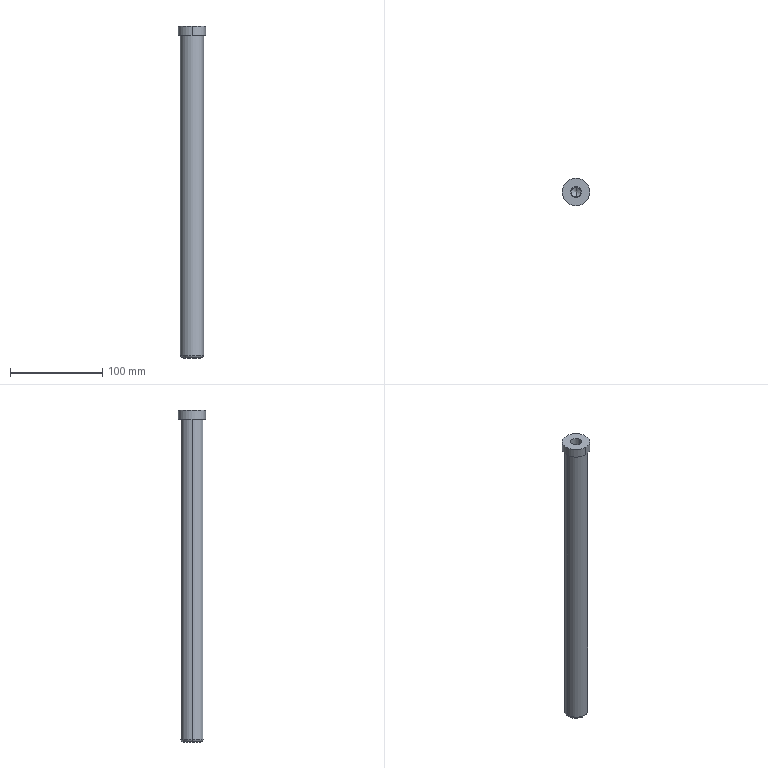Part | Creo | 1 solid | 18 faces | box 30 x 30 x 360 mm | volume 175415 mm3 | cylinder 8 | torus 4 | plane 4 | cone 2 | commonest cylinder face diameters 10.5 x2 12 x2 25 x2 30 x2
STEP:
#1=CARTESIAN_POINT('',(-230.5,220.005,-24.44));
#2=VERTEX_POINT('',#1);
#3=CARTESIAN_POINT('',(-255.5,220.005,-24.44));
#4=VERTEX_POINT('',#3);
#5=CARTESIAN_POINT('',(-243.,220.005,-24.44));
#6=DIRECTION('',(0.,0.,-1.));
#7=DIRECTION('',(1.,0.,0.));
#8=AXIS2_PLACEMENT_3D('',#5,#6,#7);
#9=CIRCLE('',#8,12.5);
#10=EDGE_CURVE('',#2,#4,#9,.T.);
#11=ORIENTED_EDGE('',*,*,#10,.T.);
#12=CARTESIAN_POINT('',(-255.5,220.005,322.56));
#13=VERTEX_POINT('',#12);
#14=CARTESIAN_POINT('',(-255.5,220.005,322.56));
#15=DIRECTION('',(0.,0.,-1.));
#16=VECTOR('',#15,347.);
#17=LINE('',#14,#16);
#18=EDGE_CURVE('',#13,#4,#17,.T.);
#19=ORIENTED_EDGE('',*,*,#18,.F.);
#20=CARTESIAN_POINT('',(-230.5,220.005,322.56));
#21=VERTEX_POINT('',#20);
#22=CARTESIAN_POINT('',(-243.,220.005,322.56));
#23=DIRECTION('',(0.,0.,1.));
#24=DIRECTION('',(-1.,0.,0.));
#25=AXIS2_PLACEMENT_3D('',#22,#23,#24);
#26=CIRCLE('',#25,12.5);
#27=EDGE_CURVE('',#13,#21,#26,.T.);
#28=ORIENTED_EDGE('',*,*,#27,.T.);
#29=CARTESIAN_POINT('',(-230.5,220.005,322.56));
#30=DIRECTION('',(0.,0.,-1.));
#31=VECTOR('',#30,347.);
#32=LINE('',#29,#31);
#33=EDGE_CURVE('',#21,#2,#32,.T.);
#34=ORIENTED_EDGE('',*,*,#33,.T.);
#35=EDGE_LOOP('',(#11,#19,#28,#34));
#36=FACE_OUTER_BOUND('',#35,.F.);
#37=CARTESIAN_POINT('',(-243.,220.005,252.56));
#38=DIRECTION('',(0.,0.,-1.));
#39=DIRECTION('',(1.,0.,0.));
#40=AXIS2_PLACEMENT_3D('',#37,#38,#39);
#41=CYLINDRICAL_SURFACE('',#40,12.5);
#42=ADVANCED_FACE('',(#36),#41,.T.);
#43=ORIENTED_EDGE('',*,*,#10,.F.);
#44=CARTESIAN_POINT('',(-231.379,220.005,-26.561));
#45=VERTEX_POINT('',#44);
#46=CARTESIAN_POINT('',(-233.5,220.005,-24.44));
#47=DIRECTION('',(0.,1.,0.));
#48=DIRECTION('',(1.,0.,0.));
#49=AXIS2_PLACEMENT_3D('',#46,#47,#48);
#50=CIRCLE('',#49,3.);
#51=EDGE_CURVE('',#2,#45,#50,.T.);
#52=ORIENTED_EDGE('',*,*,#51,.T.);
#53=CARTESIAN_POINT('',(-254.621,220.005,-26.561));
#54=VERTEX_POINT('',#53);
#55=CARTESIAN_POINT('',(-243.,220.005,-26.561));
#56=DIRECTION('',(0.,0.,-1.));
#57=DIRECTION('',(1.,0.,0.));
#58=AXIS2_PLACEMENT_3D('',#55,#56,#57);
#59=CIRCLE('',#58,11.621);
#60=EDGE_CURVE('',#45,#54,#59,.T.);
#61=ORIENTED_EDGE('',*,*,#60,.T.);
#62=CARTESIAN_POINT('',(-252.5,220.005,-24.44));
#63=DIRECTION('',(0.,-1.,0.));
#64=DIRECTION('',(-1.,0.,0.));
#65=AXIS2_PLACEMENT_3D('',#62,#63,#64);
#66=CIRCLE('',#65,3.);
#67=EDGE_CURVE('',#4,#54,#66,.T.);
#68=ORIENTED_EDGE('',*,*,#67,.F.);
#69=EDGE_LOOP('',(#43,#52,#61,#68));
#70=FACE_OUTER_BOUND('',#69,.F.);
#71=CARTESIAN_POINT('',(-243.,220.005,-24.44));
#72=DIRECTION('',(0.,0.,-1.));
#73=DIRECTION('',(-1.,0.,0.));
#74=AXIS2_PLACEMENT_3D('',#71,#72,#73);
#75=TOROIDAL_SURFACE('',#74,9.5,3.);
#76=ADVANCED_FACE('',(#70),#75,.T.);
#77=CARTESIAN_POINT('',(-243.,220.005,-24.44));
#78=DIRECTION('',(0.,0.,-1.));
#79=DIRECTION('',(-1.,0.,0.));
#80=AXIS2_PLACEMENT_3D('',#77,#78,#79);
#81=CIRCLE('',#80,12.5);
#82=EDGE_CURVE('',#4,#2,#81,.T.);
#83=ORIENTED_EDGE('',*,*,#82,.F.);
#84=ORIENTED_EDGE('',*,*,#67,.T.);
#85=CARTESIAN_POINT('',(-243.,220.005,-26.561));
#86=DIRECTION('',(0.,0.,-1.));
#87=DIRECTION('',(-1.,0.,0.));
#88=AXIS2_PLACEMENT_3D('',#85,#86,#87);
#89=CIRCLE('',#88,11.621);
#90=EDGE_CURVE('',#54,#45,#89,.T.);
#91=ORIENTED_EDGE('',*,*,#90,.T.);
#92=ORIENTED_EDGE('',*,*,#51,.F.);
#93=EDGE_LOOP('',(#83,#84,#91,#92));
#94=FACE_OUTER_BOUND('',#93,.F.);
#95=CARTESIAN_POINT('',(-243.,220.005,-24.44));
#96=DIRECTION('',(0.,0.,-1.));
#97=DIRECTION('',(-1.,0.,0.));
#98=AXIS2_PLACEMENT_3D('',#95,#96,#97);
#99=TOROIDAL_SURFACE('',#98,9.5,3.);
#100=ADVANCED_FACE('',(#94),#99,.T.);
#101=ORIENTED_EDGE('',*,*,#82,.T.);
#102=ORIENTED_EDGE('',*,*,#33,.F.);
#103=CARTESIAN_POINT('',(-243.,220.005,322.56));
#104=DIRECTION('',(0.,0.,1.));
#105=DIRECTION('',(1.,0.,0.));
#106=AXIS2_PLACEMENT_3D('',#103,#104,#105);
#107=CIRCLE('',#106,12.5);
#108=EDGE_CURVE('',#21,#13,#107,.T.);
#109=ORIENTED_EDGE('',*,*,#108,.T.);
#110=ORIENTED_EDGE('',*,*,#18,.T.);
#111=EDGE_LOOP('',(#101,#102,#109,#110));
#112=FACE_OUTER_BOUND('',#111,.F.);
#113=CARTESIAN_POINT('',(-243.,220.005,252.56));
#114=DIRECTION('',(0.,0.,-1.));
#115=DIRECTION('',(1.,0.,0.));
#116=AXIS2_PLACEMENT_3D('',#113,#114,#115);
#117=CYLINDRICAL_SURFACE('',#116,12.5);
#118=ADVANCED_FACE('',(#112),#117,.T.);
#119=CARTESIAN_POINT('',(-228.,220.005,322.56));
#120=VERTEX_POINT('',#119);
#121=CARTESIAN_POINT('',(-243.,205.005,322.56));
#122=VERTEX_POINT('',#121);
#123=CARTESIAN_POINT('',(-243.,220.005,322.56));
#124=DIRECTION('',(0.,0.,-1.));
#125=DIRECTION('',(1.,0.,0.));
#126=AXIS2_PLACEMENT_3D('',#123,#124,#125);
#127=CIRCLE('',#126,15.);
#128=EDGE_CURVE('',#120,#122,#127,.T.);
#129=ORIENTED_EDGE('',*,*,#128,.F.);
#130=CARTESIAN_POINT('',(-243.,235.005,322.56));
#131=VERTEX_POINT('',#130);
#132=CARTESIAN_POINT('',(-243.,220.005,322.56));
#133=DIRECTION('',(0.,0.,-1.));
#134=DIRECTION('',(0.,1.,0.));
#135=AXIS2_PLACEMENT_3D('',#132,#133,#134);
#136=CIRCLE('',#135,15.);
#137=EDGE_CURVE('',#131,#120,#136,.T.);
#138=ORIENTED_EDGE('',*,*,#137,.F.);
#139=CARTESIAN_POINT('',(-258.,220.005,322.56));
#140=VERTEX_POINT('',#139);
#141=CARTESIAN_POINT('',(-243.,220.005,322.56));
#142=DIRECTION('',(0.,0.,-1.));
#143=DIRECTION('',(-1.,0.,0.));
#144=AXIS2_PLACEMENT_3D('',#141,#142,#143);
#145=CIRCLE('',#144,15.);
#146=EDGE_CURVE('',#140,#131,#145,.T.);
#147=ORIENTED_EDGE('',*,*,#146,.F.);
#148=CARTESIAN_POINT('',(-243.,220.005,322.56));
#149=DIRECTION('',(0.,0.,-1.));
#150=DIRECTION('',(0.,-1.,0.));
#151=AXIS2_PLACEMENT_3D('',#148,#149,#150);
#152=CIRCLE('',#151,15.);
#153=EDGE_CURVE('',#122,#140,#152,.T.);
#154=ORIENTED_EDGE('',*,*,#153,.F.);
#155=EDGE_LOOP('',(#129,#138,#147,#154));
#156=FACE_OUTER_BOUND('',#155,.F.);
#157=ORIENTED_EDGE('',*,*,#108,.F.);
#158=ORIENTED_EDGE('',*,*,#27,.F.);
#159=EDGE_LOOP('',(#157,#158));
#160=FACE_BOUND('',#159,.F.);
#161=CARTESIAN_POINT('',(-115.,-14.995,322.56));
#162=DIRECTION('',(0.,0.,1.));
#163=DIRECTION('',(0.,-1.,0.));
#164=AXIS2_PLACEMENT_3D('',#161,#162,#163);
#165=PLANE('',#164);
#166=ADVANCED_FACE('',(#156,#160),#165,.F.);
#167=CARTESIAN_POINT('',(-228.,220.005,332.56));
#168=VERTEX_POINT('',#167);
#169=CARTESIAN_POINT('',(-243.,235.005,332.56));
#170=VERTEX_POINT('',#169);
#171=CARTESIAN_POINT('',(-243.,220.005,332.56));
#172=DIRECTION('',(0.,0.,1.));
#173=DIRECTION('',(1.,0.,0.));
#174=AXIS2_PLACEMENT_3D('',#171,#172,#173);
#175=CIRCLE('',#174,15.);
#176=EDGE_CURVE('',#168,#170,#175,.T.);
#177=ORIENTED_EDGE('',*,*,#176,.T.);
#178=CARTESIAN_POINT('',(-243.,235.005,322.56));
#179=DIRECTION('',(0.,0.,1.));
#180=VECTOR('',#179,10.);
#181=LINE('',#178,#180);
#182=EDGE_CURVE('',#131,#170,#181,.T.);
#183=ORIENTED_EDGE('',*,*,#182,.F.);
#184=ORIENTED_EDGE('',*,*,#137,.T.);
#185=ORIENTED_EDGE('',*,*,#128,.T.);
#186=CARTESIAN_POINT('',(-243.,205.005,332.56));
#187=VERTEX_POINT('',#186);
#188=CARTESIAN_POINT('',(-243.,205.005,322.56));
#189=DIRECTION('',(0.,0.,1.));
#190=VECTOR('',#189,10.);
#191=LINE('',#188,#190);
#192=EDGE_CURVE('',#122,#187,#191,.T.);
#193=ORIENTED_EDGE('',*,*,#192,.T.);
#194=CARTESIAN_POINT('',(-243.,220.005,332.56));
#195=DIRECTION('',(0.,0.,1.));
#196=DIRECTION('',(0.,-1.,0.));
#197=AXIS2_PLACEMENT_3D('',#194,#195,#196);
#198=CIRCLE('',#197,15.);
#199=EDGE_CURVE('',#187,#168,#198,.T.);
#200=ORIENTED_EDGE('',*,*,#199,.T.);
#201=EDGE_LOOP('',(#177,#183,#184,#185,#193,#200));
#202=FACE_OUTER_BOUND('',#201,.F.);
#203=CARTESIAN_POINT('',(-243.,220.005,257.56));
#204=DIRECTION('',(0.,0.,1.));
#205=DIRECTION('',(0.,-1.,0.));
#206=AXIS2_PLACEMENT_3D('',#203,#204,#205);
#207=CYLINDRICAL_SURFACE('',#206,15.);
#208=ADVANCED_FACE('',(#202),#207,.T.);
#209=CARTESIAN_POINT('',(-258.,220.005,332.56));
#210=VERTEX_POINT('',#209);
#211=CARTESIAN_POINT('',(-243.,220.005,332.56));
#212=DIRECTION('',(0.,0.,1.));
#213=DIRECTION('',(-1.,0.,0.));
#214=AXIS2_PLACEMENT_3D('',#211,#212,#213);
#215=CIRCLE('',#214,15.);
#216=EDGE_CURVE('',#210,#187,#215,.T.);
#217=ORIENTED_EDGE('',*,*,#216,.F.);
#218=CARTESIAN_POINT('',(-243.,220.005,332.56));
#219=DIRECTION('',(0.,0.,1.));
#220=DIRECTION('',(0.,1.,0.));
#221=AXIS2_PLACEMENT_3D('',#218,#219,#220);
#222=CIRCLE('',#221,15.);
#223=EDGE_CURVE('',#170,#210,#222,.T.);
#224=ORIENTED_EDGE('',*,*,#223,.F.);
#225=ORIENTED_EDGE('',*,*,#176,.F.);
#226=ORIENTED_EDGE('',*,*,#199,.F.);
#227=EDGE_LOOP('',(#217,#224,#225,#226));
#228=FACE_OUTER_BOUND('',#227,.F.);
#229=CARTESIAN_POINT('',(-249.,220.005,332.56));
#230=VERTEX_POINT('',#229);
#231=CARTESIAN_POINT('',(-237.,220.005,332.56));
#232=VERTEX_POINT('',#231);
#233=CARTESIAN_POINT('',(-243.,220.005,332.56));
#234=DIRECTION('',(0.,0.,-1.));
#235=DIRECTION('',(-1.,0.,0.));
#236=AXIS2_PLACEMENT_3D('',#233,#234,#235);
#237=CIRCLE('',#236,6.);
#238=EDGE_CURVE('',#230,#232,#237,.T.);
#239=ORIENTED_EDGE('',*,*,#238,.F.);
#240=CARTESIAN_POINT('',(-243.,220.005,332.56));
#241=DIRECTION('',(0.,0.,-1.));
#242=DIRECTION('',(1.,0.,0.));
#243=AXIS2_PLACEMENT_3D('',#240,#241,#242);
#244=CIRCLE('',#243,6.);
#245=EDGE_CURVE('',#232,#230,#244,.T.);
#246=ORIENTED_EDGE('',*,*,#245,.F.);
#247=EDGE_LOOP('',(#239,#246));
#248=FACE_BOUND('',#247,.F.);
#249=CARTESIAN_POINT('',(-115.,-14.995,332.56));
#250=DIRECTION('',(0.,0.,-1.));
#251=DIRECTION('',(1.,0.,0.));
#252=AXIS2_PLACEMENT_3D('',#249,#250,#251);
#253=PLANE('',#252);
#254=ADVANCED_FACE('',(#228,#248),#253,.F.);
#255=ORIENTED_EDGE('',*,*,#238,.T.);
#256=CARTESIAN_POINT('',(-237.,220.005,310.56));
#257=VERTEX_POINT('',#256);
#258=CARTESIAN_POINT('',(-237.,220.005,332.56));
#259=DIRECTION('',(0.,0.,-1.));
#260=VECTOR('',#259,22.);
#261=LINE('',#258,#260);
#262=EDGE_CURVE('',#232,#257,#261,.T.);
#263=ORIENTED_EDGE('',*,*,#262,.T.);
#264=CARTESIAN_POINT('',(-249.,220.005,310.56));
#265=VERTEX_POINT('',#264);
#266=CARTESIAN_POINT('',(-243.,220.005,310.56));
#267=DIRECTION('',(0.,0.,1.));
#268=DIRECTION('',(1.,0.,0.));
#269=AXIS2_PLACEMENT_3D('',#266,#267,#268);
#270=CIRCLE('',#269,6.);
#271=EDGE_CURVE('',#257,#265,#270,.T.);
#272=ORIENTED_EDGE('',*,*,#271,.T.);
#273=CARTESIAN_POINT('',(-249.,220.005,332.56));
#274=DIRECTION('',(0.,0.,-1.));
#275=VECTOR('',#274,22.);
#276=LINE('',#273,#275);
#277=EDGE_CURVE('',#230,#265,#276,.T.);
#278=ORIENTED_EDGE('',*,*,#277,.F.);
#279=EDGE_LOOP('',(#255,#263,#272,#278));
#280=FACE_OUTER_BOUND('',#279,.F.);
#281=CARTESIAN_POINT('',(-243.,220.005,345.56));
#282=DIRECTION('',(0.,0.,-1.));
#283=DIRECTION('',(-1.,0.,0.));
#284=AXIS2_PLACEMENT_3D('',#281,#282,#283);
#285=CYLINDRICAL_SURFACE('',#284,6.);
#286=ADVANCED_FACE('',(#280),#285,.F.);
#287=ORIENTED_EDGE('',*,*,#245,.T.);
#288=ORIENTED_EDGE('',*,*,#277,.T.);
#289=CARTESIAN_POINT('',(-243.,220.005,310.56));
#290=DIRECTION('',(0.,0.,1.));
#291=DIRECTION('',(-1.,0.,0.));
#292=AXIS2_PLACEMENT_3D('',#289,#290,#291);
#293=CIRCLE('',#292,6.);
#294=EDGE_CURVE('',#265,#257,#293,.T.);
#295=ORIENTED_EDGE('',*,*,#294,.T.);
#296=ORIENTED_EDGE('',*,*,#262,.F.);
#297=EDGE_LOOP('',(#287,#288,#295,#296));
#298=FACE_OUTER_BOUND('',#297,.F.);
#299=CARTESIAN_POINT('',(-243.,220.005,345.56));
#300=DIRECTION('',(0.,0.,-1.));
#301=DIRECTION('',(-1.,0.,0.));
#302=AXIS2_PLACEMENT_3D('',#299,#300,#301);
#303=CYLINDRICAL_SURFACE('',#302,6.);
#304=ADVANCED_FACE('',(#298),#303,.F.);
#305=ORIENTED_EDGE('',*,*,#294,.F.);
#306=ORIENTED_EDGE('',*,*,#271,.F.);
#307=EDGE_LOOP('',(#305,#306));
#308=FACE_OUTER_BOUND('',#307,.F.);
#309=CARTESIAN_POINT('',(-248.25,220.005,310.56));
#310=VERTEX_POINT('',#309);
#311=CARTESIAN_POINT('',(-237.75,220.005,310.56));
#312=VERTEX_POINT('',#311);
#313=CARTESIAN_POINT('',(-243.,220.005,310.56));
#314=DIRECTION('',(0.,0.,-1.));
#315=DIRECTION('',(-1.,0.,0.));
#316=AXIS2_PLACEMENT_3D('',#313,#314,#315);
#317=CIRCLE('',#316,5.25);
#318=EDGE_CURVE('',#310,#312,#317,.T.);
#319=ORIENTED_EDGE('',*,*,#318,.F.);
#320=CARTESIAN_POINT('',(-243.,220.005,310.56));
#321=DIRECTION('',(0.,0.,-1.));
#322=DIRECTION('',(1.,0.,0.));
#323=AXIS2_PLACEMENT_3D('',#320,#321,#322);
#324=CIRCLE('',#323,5.25);
#325=EDGE_CURVE('',#312,#310,#324,.T.);
#326=ORIENTED_EDGE('',*,*,#325,.F.);
#327=EDGE_LOOP('',(#319,#326));
#328=FACE_BOUND('',#327,.F.);
#329=CARTESIAN_POINT('',(-243.,220.005,310.56));
#330=DIRECTION('',(0.,0.,-1.));
#331=DIRECTION('',(-1.,0.,0.));
#332=AXIS2_PLACEMENT_3D('',#329,#330,#331);
#333=PLANE('',#332);
#334=ADVANCED_FACE('',(#308,#328),#333,.F.);
#335=ORIENTED_EDGE('',*,*,#318,.T.);
#336=CARTESIAN_POINT('',(-237.75,220.005,302.05));
#337=VERTEX_POINT('',#336);
#338=CARTESIAN_POINT('',(-237.75,220.005,310.56));
#339=DIRECTION('',(0.,0.,-1.));
#340=VECTOR('',#339,8.51);
#341=LINE('',#338,#340);
#342=EDGE_CURVE('',#312,#337,#341,.T.);
#343=ORIENTED_EDGE('',*,*,#342,.T.);
#344=CARTESIAN_POINT('',(-243.,225.255,302.05));
#345=VERTEX_POINT('',#344);
#346=CARTESIAN_POINT('',(-243.,220.005,302.05));
#347=DIRECTION('',(0.,0.,1.));
#348=DIRECTION('',(1.,0.,0.));
#349=AXIS2_PLACEMENT_3D('',#346,#347,#348);
#350=CIRCLE('',#349,5.25);
#351=EDGE_CURVE('',#337,#345,#350,.T.);
#352=ORIENTED_EDGE('',*,*,#351,.T.);
#353=CARTESIAN_POINT('',(-248.25,220.005,302.05));
#354=VERTEX_POINT('',#353);
#355=CARTESIAN_POINT('',(-243.,220.005,302.05));
#356=DIRECTION('',(0.,0.,1.));
#357=DIRECTION('',(0.,1.,0.));
#358=AXIS2_PLACEMENT_3D('',#355,#356,#357);
#359=CIRCLE('',#358,5.25);
#360=EDGE_CURVE('',#345,#354,#359,.T.);
#361=ORIENTED_EDGE('',*,*,#360,.T.);
#362=CARTESIAN_POINT('',(-248.25,220.005,310.56));
#363=DIRECTION('',(0.,0.,-1.));
#364=VECTOR('',#363,8.51);
#365=LINE('',#362,#364);
#366=EDGE_CURVE('',#310,#354,#365,.T.);
#367=ORIENTED_EDGE('',*,*,#366,.F.);
#368=EDGE_LOOP('',(#335,#343,#352,#361,#367));
#369=FACE_OUTER_BOUND('',#368,.F.);
#370=CARTESIAN_POINT('',(-243.,220.005,345.56));
#371=DIRECTION('',(0.,0.,-1.));
#372=DIRECTION('',(-1.,0.,0.));
#373=AXIS2_PLACEMENT_3D('',#370,#371,#372);
#374=CYLINDRICAL_SURFACE('',#373,5.25);
#375=ADVANCED_FACE('',(#369),#374,.F.);
#376=ORIENTED_EDGE('',*,*,#325,.T.);
#377=ORIENTED_EDGE('',*,*,#366,.T.);
#378=CARTESIAN_POINT('',(-243.,214.755,302.05));
#379=VERTEX_POINT('',#378);
#380=CARTESIAN_POINT('',(-243.,220.005,302.05));
#381=DIRECTION('',(0.,0.,1.));
#382=DIRECTION('',(-1.,0.,0.));
#383=AXIS2_PLACEMENT_3D('',#380,#381,#382);
#384=CIRCLE('',#383,5.25);
#385=EDGE_CURVE('',#354,#379,#384,.T.);
#386=ORIENTED_EDGE('',*,*,#385,.T.);
#387=CARTESIAN_POINT('',(-243.,220.005,302.05));
#388=DIRECTION('',(0.,0.,1.));
#389=DIRECTION('',(0.,-1.,0.));
#390=AXIS2_PLACEMENT_3D('',#387,#388,#389);
#391=CIRCLE('',#390,5.25);
#392=EDGE_CURVE('',#379,#337,#391,.T.);
#393=ORIENTED_EDGE('',*,*,#392,.T.);
#394=ORIENTED_EDGE('',*,*,#342,.F.);
#395=EDGE_LOOP('',(#376,#377,#386,#393,#394));
#396=FACE_OUTER_BOUND('',#395,.F.);
#397=CARTESIAN_POINT('',(-243.,220.005,345.56));
#398=DIRECTION('',(0.,0.,-1.));
#399=DIRECTION('',(-1.,0.,0.));
#400=AXIS2_PLACEMENT_3D('',#397,#398,#399);
#401=CYLINDRICAL_SURFACE('',#400,5.25);
#402=ADVANCED_FACE('',(#396),#401,.F.);
#403=ORIENTED_EDGE('',*,*,#360,.F.);
#404=CARTESIAN_POINT('',(-243.,220.005,298.896));
#405=VERTEX_POINT('',#404);
#406=CARTESIAN_POINT('',(-243.,220.005,298.896));
#407=DIRECTION('',(0.,0.8572,0.515));
#408=VECTOR('',#407,6.125);
#409=LINE('',#406,#408);
#410=EDGE_CURVE('',#405,#345,#409,.T.);
#411=ORIENTED_EDGE('',*,*,#410,.F.);
#412=CARTESIAN_POINT('',(-243.,220.005,298.896));
#413=DIRECTION('',(0.,-0.8572,0.515));
#414=VECTOR('',#413,6.125);
#415=LINE('',#412,#414);
#416=EDGE_CURVE('',#405,#379,#415,.T.);
#417=ORIENTED_EDGE('',*,*,#416,.T.);
#418=ORIENTED_EDGE('',*,*,#385,.F.);
#419=EDGE_LOOP('',(#403,#411,#417,#418));
#420=FACE_OUTER_BOUND('',#419,.F.);
#421=CARTESIAN_POINT('',(-243.,220.005,300.585));
#422=DIRECTION('',(0.,0.,1.));
#423=DIRECTION('',(0.,1.,0.));
#424=AXIS2_PLACEMENT_3D('',#421,#422,#423);
#425=CONICAL_SURFACE('',#424,2.811,59.);
#426=ADVANCED_FACE('',(#420),#425,.F.);
#427=ORIENTED_EDGE('',*,*,#351,.F.);
#428=ORIENTED_EDGE('',*,*,#392,.F.);
#429=ORIENTED_EDGE('',*,*,#416,.F.);
#430=ORIENTED_EDGE('',*,*,#410,.T.);
#431=EDGE_LOOP('',(#427,#428,#429,#430));
#432=FACE_OUTER_BOUND('',#431,.F.);
#433=CARTESIAN_POINT('',(-243.,220.005,300.585));
#434=DIRECTION('',(0.,0.,1.));
#435=DIRECTION('',(0.,1.,0.));
#436=AXIS2_PLACEMENT_3D('',#433,#434,#435);
#437=CONICAL_SURFACE('',#436,2.811,59.);
#438=ADVANCED_FACE('',(#432),#437,.F.);
#439=ORIENTED_EDGE('',*,*,#223,.T.);
#440=ORIENTED_EDGE('',*,*,#216,.T.);
#441=ORIENTED_EDGE('',*,*,#192,.F.);
#442=ORIENTED_EDGE('',*,*,#153,.T.);
#443=ORIENTED_EDGE('',*,*,#146,.T.);
#444=ORIENTED_EDGE('',*,*,#182,.T.);
#445=EDGE_LOOP('',(#439,#440,#441,#442,#443,#444));
#446=FACE_OUTER_BOUND('',#445,.F.);
#447=CARTESIAN_POINT('',(-243.,220.005,257.56));
#448=DIRECTION('',(0.,0.,1.));
#449=DIRECTION('',(0.,-1.,0.));
#450=AXIS2_PLACEMENT_3D('',#447,#448,#449);
#451=CYLINDRICAL_SURFACE('',#450,15.);
#452=ADVANCED_FACE('',(#446),#451,.T.);
#453=CARTESIAN_POINT('',(-252.5,220.005,-27.44));
#454=VERTEX_POINT('',#453);
#455=CARTESIAN_POINT('',(-233.5,220.005,-27.44));
#456=VERTEX_POINT('',#455);
#457=CARTESIAN_POINT('',(-243.,220.005,-27.44));
#458=DIRECTION('',(0.,0.,-1.));
#459=DIRECTION('',(-1.,0.,0.));
#460=AXIS2_PLACEMENT_3D('',#457,#458,#459);
#461=CIRCLE('',#460,9.5);
#462=EDGE_CURVE('',#454,#456,#461,.T.);
#463=ORIENTED_EDGE('',*,*,#462,.T.);
#464=CARTESIAN_POINT('',(-233.5,220.005,-24.44));
#465=DIRECTION('',(0.,1.,0.));
#466=DIRECTION('',(0.7071,0.,-0.7071));
#467=AXIS2_PLACEMENT_3D('',#464,#465,#466);
#468=CIRCLE('',#467,3.);
#469=EDGE_CURVE('',#45,#456,#468,.T.);
#470=ORIENTED_EDGE('',*,*,#469,.F.);
#471=ORIENTED_EDGE('',*,*,#90,.F.);
#472=CARTESIAN_POINT('',(-252.5,220.005,-24.44));
#473=DIRECTION('',(0.,-1.,0.));
#474=DIRECTION('',(-0.7071,0.,-0.7071));
#475=AXIS2_PLACEMENT_3D('',#472,#473,#474);
#476=CIRCLE('',#475,3.);
#477=EDGE_CURVE('',#54,#454,#476,.T.);
#478=ORIENTED_EDGE('',*,*,#477,.T.);
#479=EDGE_LOOP('',(#463,#470,#471,#478));
#480=FACE_OUTER_BOUND('',#479,.F.);
#481=CARTESIAN_POINT('',(-243.,220.005,-24.44));
#482=DIRECTION('',(0.,0.,-1.));
#483=DIRECTION('',(-1.,0.,0.));
#484=AXIS2_PLACEMENT_3D('',#481,#482,#483);
#485=TOROIDAL_SURFACE('',#484,9.5,3.);
#486=ADVANCED_FACE('',(#480),#485,.T.);
#487=ORIENTED_EDGE('',*,*,#462,.F.);
#488=CARTESIAN_POINT('',(-243.,220.005,-27.44));
#489=DIRECTION('',(0.,0.,-1.));
#490=DIRECTION('',(1.,0.,0.));
#491=AXIS2_PLACEMENT_3D('',#488,#489,#490);
#492=CIRCLE('',#491,9.5);
#493=EDGE_CURVE('',#456,#454,#492,.T.);
#494=ORIENTED_EDGE('',*,*,#493,.F.);
#495=EDGE_LOOP('',(#487,#494));
#496=FACE_OUTER_BOUND('',#495,.F.);
#497=CARTESIAN_POINT('',(-288.,-14.995,-27.44));
#498=DIRECTION('',(0.,0.,-1.));
#499=DIRECTION('',(-1.,0.,0.));
#500=AXIS2_PLACEMENT_3D('',#497,#498,#499);
#501=PLANE('',#500);
#502=ADVANCED_FACE('',(#496),#501,.T.);
#503=ORIENTED_EDGE('',*,*,#493,.T.);
#504=ORIENTED_EDGE('',*,*,#477,.F.);
#505=ORIENTED_EDGE('',*,*,#60,.F.);
#506=ORIENTED_EDGE('',*,*,#469,.T.);
#507=EDGE_LOOP('',(#503,#504,#505,#506));
#508=FACE_OUTER_BOUND('',#507,.F.);
#509=CARTESIAN_POINT('',(-243.,220.005,-24.44));
#510=DIRECTION('',(0.,0.,-1.));
#511=DIRECTION('',(-1.,0.,0.));
#512=AXIS2_PLACEMENT_3D('',#509,#510,#511);
#513=TOROIDAL_SURFACE('',#512,9.5,3.);
#514=ADVANCED_FACE('',(#508),#513,.T.);
#515=CLOSED_SHELL('',(#42,#76,#100,#118,#166,#208,#254,#286,#304,#334,#375,#402,#426,#438,#452,#486,#502,#514));
#516=MANIFOLD_SOLID_BREP('',#515);
#517=(LENGTH_UNIT()NAMED_UNIT(*)SI_UNIT(.MILLI.,.METRE.));
#518=UNCERTAINTY_MEASURE_WITH_UNIT(LENGTH_MEASURE(0.03625),#517,'','');
#519=(NAMED_UNIT(*)PLANE_ANGLE_UNIT()SI_UNIT($,.RADIAN.));
#520=PLANE_ANGLE_MEASURE_WITH_UNIT(PLANE_ANGLE_MEASURE(0.01745),#519);
#521=(CONVERSION_BASED_UNIT('DEGREE',#520)NAMED_UNIT(*)PLANE_ANGLE_UNIT());
#522=(NAMED_UNIT(*)SI_UNIT($,.STERADIAN.)SOLID_ANGLE_UNIT());
#523=(GEOMETRIC_REPRESENTATION_CONTEXT(3)GLOBAL_UNCERTAINTY_ASSIGNED_CONTEXT((#518))GLOBAL_UNIT_ASSIGNED_CONTEXT((#517,#521,#522))REPRESENTATION_CONTEXT('',''));
#524=ADVANCED_BREP_SHAPE_REPRESENTATION('',(#516),#523);